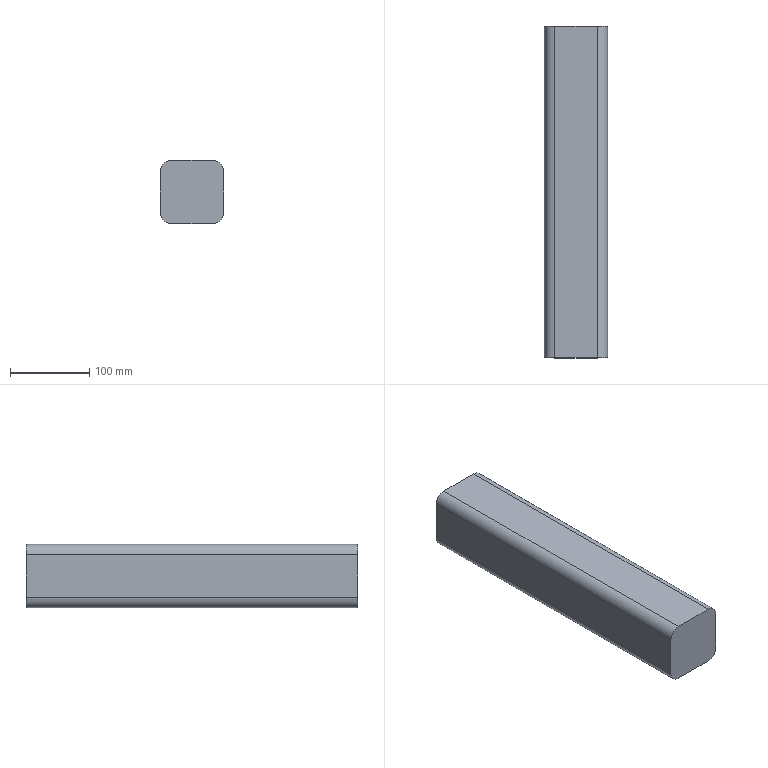Part | SolidWorks | features Extrusion 1 | 1 solid | 10 faces | box 80 x 420 x 80 mm | volume 2623906 mm3 | plane 6 | cylinder 4 | commonest cylinder face diameters 26.667 x4
STEP:
#1=CARTESIAN_POINT('',(26.667,0.,-40.));
#2=VERTEX_POINT('',#1);
#3=CARTESIAN_POINT('',(40.,0.,-26.667));
#4=VERTEX_POINT('',#3);
#5=CARTESIAN_POINT('',(26.667,0.,-26.667));
#6=DIRECTION('',(0.,-1.,0.));
#7=DIRECTION('',(0.,0.,-1.));
#8=AXIS2_PLACEMENT_3D('',#5,#6,#7);
#9=CIRCLE('',#8,13.333);
#10=EDGE_CURVE('',#2,#4,#9,.T.);
#11=ORIENTED_EDGE('',*,*,#10,.F.);
#12=CARTESIAN_POINT('',(26.667,420.,-40.));
#13=VERTEX_POINT('',#12);
#14=CARTESIAN_POINT('',(26.667,420.,-40.));
#15=DIRECTION('',(0.,-1.,0.));
#16=VECTOR('',#15,1000.);
#17=LINE('',#14,#16);
#18=EDGE_CURVE('',#13,#2,#17,.T.);
#19=ORIENTED_EDGE('',*,*,#18,.F.);
#20=CARTESIAN_POINT('',(40.,420.,-26.667));
#21=VERTEX_POINT('',#20);
#22=CARTESIAN_POINT('',(26.667,420.,-26.667));
#23=DIRECTION('',(0.,-1.,0.));
#24=DIRECTION('',(0.,0.,-1.));
#25=AXIS2_PLACEMENT_3D('',#22,#23,#24);
#26=CIRCLE('',#25,13.333);
#27=EDGE_CURVE('',#13,#21,#26,.T.);
#28=ORIENTED_EDGE('',*,*,#27,.T.);
#29=CARTESIAN_POINT('',(40.,420.,-26.667));
#30=DIRECTION('',(0.,-1.,0.));
#31=VECTOR('',#30,1000.);
#32=LINE('',#29,#31);
#33=EDGE_CURVE('',#21,#4,#32,.T.);
#34=ORIENTED_EDGE('',*,*,#33,.T.);
#35=EDGE_LOOP('',(#11,#19,#28,#34));
#36=FACE_OUTER_BOUND('',#35,.T.);
#37=CARTESIAN_POINT('',(26.667,420.,-26.667));
#38=DIRECTION('',(0.,-1.,0.));
#39=DIRECTION('',(0.,0.,-1.));
#40=AXIS2_PLACEMENT_3D('',#37,#38,#39);
#41=CYLINDRICAL_SURFACE('',#40,13.333);
#42=ADVANCED_FACE('',(#36),#41,.T.);
#43=CARTESIAN_POINT('',(-26.667,0.,-40.));
#44=VERTEX_POINT('',#43);
#45=CARTESIAN_POINT('',(-26.667,0.,-40.));
#46=DIRECTION('',(1.,0.,0.));
#47=VECTOR('',#46,1000.);
#48=LINE('',#45,#47);
#49=EDGE_CURVE('',#44,#2,#48,.T.);
#50=ORIENTED_EDGE('',*,*,#49,.F.);
#51=CARTESIAN_POINT('',(-26.667,420.,-40.));
#52=VERTEX_POINT('',#51);
#53=CARTESIAN_POINT('',(-26.667,420.,-40.));
#54=DIRECTION('',(0.,-1.,0.));
#55=VECTOR('',#54,1000.);
#56=LINE('',#53,#55);
#57=EDGE_CURVE('',#52,#44,#56,.T.);
#58=ORIENTED_EDGE('',*,*,#57,.F.);
#59=CARTESIAN_POINT('',(-26.667,420.,-40.));
#60=DIRECTION('',(1.,0.,0.));
#61=VECTOR('',#60,1000.);
#62=LINE('',#59,#61);
#63=EDGE_CURVE('',#52,#13,#62,.T.);
#64=ORIENTED_EDGE('',*,*,#63,.T.);
#65=ORIENTED_EDGE('',*,*,#18,.T.);
#66=EDGE_LOOP('',(#50,#58,#64,#65));
#67=FACE_OUTER_BOUND('',#66,.T.);
#68=CARTESIAN_POINT('',(-26.667,420.,-40.));
#69=DIRECTION('',(0.,0.,-1.));
#70=DIRECTION('',(0.,1.,0.));
#71=AXIS2_PLACEMENT_3D('',#68,#69,#70);
#72=PLANE('',#71);
#73=ADVANCED_FACE('',(#67),#72,.T.);
#74=CARTESIAN_POINT('',(-40.,0.,-26.667));
#75=VERTEX_POINT('',#74);
#76=CARTESIAN_POINT('',(-26.667,0.,-26.667));
#77=DIRECTION('',(0.,-1.,0.));
#78=DIRECTION('',(0.,0.,-1.));
#79=AXIS2_PLACEMENT_3D('',#76,#77,#78);
#80=CIRCLE('',#79,13.333);
#81=EDGE_CURVE('',#75,#44,#80,.T.);
#82=ORIENTED_EDGE('',*,*,#81,.F.);
#83=CARTESIAN_POINT('',(-40.,420.,-26.667));
#84=VERTEX_POINT('',#83);
#85=CARTESIAN_POINT('',(-40.,420.,-26.667));
#86=DIRECTION('',(0.,-1.,0.));
#87=VECTOR('',#86,1000.);
#88=LINE('',#85,#87);
#89=EDGE_CURVE('',#84,#75,#88,.T.);
#90=ORIENTED_EDGE('',*,*,#89,.F.);
#91=CARTESIAN_POINT('',(-26.667,420.,-26.667));
#92=DIRECTION('',(0.,-1.,0.));
#93=DIRECTION('',(0.,0.,-1.));
#94=AXIS2_PLACEMENT_3D('',#91,#92,#93);
#95=CIRCLE('',#94,13.333);
#96=EDGE_CURVE('',#84,#52,#95,.T.);
#97=ORIENTED_EDGE('',*,*,#96,.T.);
#98=ORIENTED_EDGE('',*,*,#57,.T.);
#99=EDGE_LOOP('',(#82,#90,#97,#98));
#100=FACE_OUTER_BOUND('',#99,.T.);
#101=CARTESIAN_POINT('',(-26.667,420.,-26.667));
#102=DIRECTION('',(0.,-1.,0.));
#103=DIRECTION('',(0.,0.,-1.));
#104=AXIS2_PLACEMENT_3D('',#101,#102,#103);
#105=CYLINDRICAL_SURFACE('',#104,13.333);
#106=ADVANCED_FACE('',(#100),#105,.T.);
#107=CARTESIAN_POINT('',(-40.,0.,26.667));
#108=VERTEX_POINT('',#107);
#109=CARTESIAN_POINT('',(-40.,0.,26.667));
#110=DIRECTION('',(0.,0.,-1.));
#111=VECTOR('',#110,1000.);
#112=LINE('',#109,#111);
#113=EDGE_CURVE('',#108,#75,#112,.T.);
#114=ORIENTED_EDGE('',*,*,#113,.F.);
#115=CARTESIAN_POINT('',(-40.,420.,26.667));
#116=VERTEX_POINT('',#115);
#117=CARTESIAN_POINT('',(-40.,420.,26.667));
#118=DIRECTION('',(0.,-1.,0.));
#119=VECTOR('',#118,1000.);
#120=LINE('',#117,#119);
#121=EDGE_CURVE('',#116,#108,#120,.T.);
#122=ORIENTED_EDGE('',*,*,#121,.F.);
#123=CARTESIAN_POINT('',(-40.,420.,26.667));
#124=DIRECTION('',(0.,0.,-1.));
#125=VECTOR('',#124,1000.);
#126=LINE('',#123,#125);
#127=EDGE_CURVE('',#116,#84,#126,.T.);
#128=ORIENTED_EDGE('',*,*,#127,.T.);
#129=ORIENTED_EDGE('',*,*,#89,.T.);
#130=EDGE_LOOP('',(#114,#122,#128,#129));
#131=FACE_OUTER_BOUND('',#130,.T.);
#132=CARTESIAN_POINT('',(-40.,420.,26.667));
#133=DIRECTION('',(-1.,0.,0.));
#134=DIRECTION('',(0.,0.,1.));
#135=AXIS2_PLACEMENT_3D('',#132,#133,#134);
#136=PLANE('',#135);
#137=ADVANCED_FACE('',(#131),#136,.T.);
#138=CARTESIAN_POINT('',(-26.667,0.,40.));
#139=VERTEX_POINT('',#138);
#140=CARTESIAN_POINT('',(-26.667,0.,26.667));
#141=DIRECTION('',(0.,-1.,0.));
#142=DIRECTION('',(0.,0.,-1.));
#143=AXIS2_PLACEMENT_3D('',#140,#141,#142);
#144=CIRCLE('',#143,13.333);
#145=EDGE_CURVE('',#139,#108,#144,.T.);
#146=ORIENTED_EDGE('',*,*,#145,.F.);
#147=CARTESIAN_POINT('',(-26.667,420.,40.));
#148=VERTEX_POINT('',#147);
#149=CARTESIAN_POINT('',(-26.667,420.,40.));
#150=DIRECTION('',(0.,-1.,0.));
#151=VECTOR('',#150,1000.);
#152=LINE('',#149,#151);
#153=EDGE_CURVE('',#148,#139,#152,.T.);
#154=ORIENTED_EDGE('',*,*,#153,.F.);
#155=CARTESIAN_POINT('',(-26.667,420.,26.667));
#156=DIRECTION('',(0.,-1.,0.));
#157=DIRECTION('',(0.,0.,-1.));
#158=AXIS2_PLACEMENT_3D('',#155,#156,#157);
#159=CIRCLE('',#158,13.333);
#160=EDGE_CURVE('',#148,#116,#159,.T.);
#161=ORIENTED_EDGE('',*,*,#160,.T.);
#162=ORIENTED_EDGE('',*,*,#121,.T.);
#163=EDGE_LOOP('',(#146,#154,#161,#162));
#164=FACE_OUTER_BOUND('',#163,.T.);
#165=CARTESIAN_POINT('',(-26.667,420.,26.667));
#166=DIRECTION('',(0.,-1.,0.));
#167=DIRECTION('',(0.,0.,-1.));
#168=AXIS2_PLACEMENT_3D('',#165,#166,#167);
#169=CYLINDRICAL_SURFACE('',#168,13.333);
#170=ADVANCED_FACE('',(#164),#169,.T.);
#171=CARTESIAN_POINT('',(26.667,0.,40.));
#172=VERTEX_POINT('',#171);
#173=CARTESIAN_POINT('',(26.667,0.,40.));
#174=DIRECTION('',(-1.,0.,0.));
#175=VECTOR('',#174,1000.);
#176=LINE('',#173,#175);
#177=EDGE_CURVE('',#172,#139,#176,.T.);
#178=ORIENTED_EDGE('',*,*,#177,.F.);
#179=CARTESIAN_POINT('',(26.667,420.,40.));
#180=VERTEX_POINT('',#179);
#181=CARTESIAN_POINT('',(26.667,420.,40.));
#182=DIRECTION('',(0.,-1.,0.));
#183=VECTOR('',#182,1000.);
#184=LINE('',#181,#183);
#185=EDGE_CURVE('',#180,#172,#184,.T.);
#186=ORIENTED_EDGE('',*,*,#185,.F.);
#187=CARTESIAN_POINT('',(26.667,420.,40.));
#188=DIRECTION('',(-1.,0.,0.));
#189=VECTOR('',#188,1000.);
#190=LINE('',#187,#189);
#191=EDGE_CURVE('',#180,#148,#190,.T.);
#192=ORIENTED_EDGE('',*,*,#191,.T.);
#193=ORIENTED_EDGE('',*,*,#153,.T.);
#194=EDGE_LOOP('',(#178,#186,#192,#193));
#195=FACE_OUTER_BOUND('',#194,.T.);
#196=CARTESIAN_POINT('',(26.667,420.,40.));
#197=DIRECTION('',(0.,0.,1.));
#198=DIRECTION('',(0.,-1.,0.));
#199=AXIS2_PLACEMENT_3D('',#196,#197,#198);
#200=PLANE('',#199);
#201=ADVANCED_FACE('',(#195),#200,.T.);
#202=CARTESIAN_POINT('',(40.,0.,26.667));
#203=VERTEX_POINT('',#202);
#204=CARTESIAN_POINT('',(26.667,0.,26.667));
#205=DIRECTION('',(0.,-1.,0.));
#206=DIRECTION('',(0.,0.,-1.));
#207=AXIS2_PLACEMENT_3D('',#204,#205,#206);
#208=CIRCLE('',#207,13.333);
#209=EDGE_CURVE('',#203,#172,#208,.T.);
#210=ORIENTED_EDGE('',*,*,#209,.F.);
#211=CARTESIAN_POINT('',(40.,420.,26.667));
#212=VERTEX_POINT('',#211);
#213=CARTESIAN_POINT('',(40.,420.,26.667));
#214=DIRECTION('',(0.,-1.,0.));
#215=VECTOR('',#214,1000.);
#216=LINE('',#213,#215);
#217=EDGE_CURVE('',#212,#203,#216,.T.);
#218=ORIENTED_EDGE('',*,*,#217,.F.);
#219=CARTESIAN_POINT('',(26.667,420.,26.667));
#220=DIRECTION('',(0.,-1.,0.));
#221=DIRECTION('',(0.,0.,-1.));
#222=AXIS2_PLACEMENT_3D('',#219,#220,#221);
#223=CIRCLE('',#222,13.333);
#224=EDGE_CURVE('',#212,#180,#223,.T.);
#225=ORIENTED_EDGE('',*,*,#224,.T.);
#226=ORIENTED_EDGE('',*,*,#185,.T.);
#227=EDGE_LOOP('',(#210,#218,#225,#226));
#228=FACE_OUTER_BOUND('',#227,.T.);
#229=CARTESIAN_POINT('',(26.667,420.,26.667));
#230=DIRECTION('',(0.,-1.,0.));
#231=DIRECTION('',(0.,0.,-1.));
#232=AXIS2_PLACEMENT_3D('',#229,#230,#231);
#233=CYLINDRICAL_SURFACE('',#232,13.333);
#234=ADVANCED_FACE('',(#228),#233,.T.);
#235=CARTESIAN_POINT('',(40.,0.,-26.667));
#236=DIRECTION('',(0.,0.,1.));
#237=VECTOR('',#236,1000.);
#238=LINE('',#235,#237);
#239=EDGE_CURVE('',#4,#203,#238,.T.);
#240=ORIENTED_EDGE('',*,*,#239,.F.);
#241=ORIENTED_EDGE('',*,*,#33,.F.);
#242=CARTESIAN_POINT('',(40.,420.,-26.667));
#243=DIRECTION('',(0.,0.,1.));
#244=VECTOR('',#243,1000.);
#245=LINE('',#242,#244);
#246=EDGE_CURVE('',#21,#212,#245,.T.);
#247=ORIENTED_EDGE('',*,*,#246,.T.);
#248=ORIENTED_EDGE('',*,*,#217,.T.);
#249=EDGE_LOOP('',(#240,#241,#247,#248));
#250=FACE_OUTER_BOUND('',#249,.T.);
#251=CARTESIAN_POINT('',(40.,420.,-26.667));
#252=DIRECTION('',(1.,0.,0.));
#253=DIRECTION('',(0.,0.,-1.));
#254=AXIS2_PLACEMENT_3D('',#251,#252,#253);
#255=PLANE('',#254);
#256=ADVANCED_FACE('',(#250),#255,.T.);
#257=ORIENTED_EDGE('',*,*,#27,.F.);
#258=ORIENTED_EDGE('',*,*,#63,.F.);
#259=ORIENTED_EDGE('',*,*,#96,.F.);
#260=ORIENTED_EDGE('',*,*,#127,.F.);
#261=ORIENTED_EDGE('',*,*,#160,.F.);
#262=ORIENTED_EDGE('',*,*,#191,.F.);
#263=ORIENTED_EDGE('',*,*,#224,.F.);
#264=ORIENTED_EDGE('',*,*,#246,.F.);
#265=EDGE_LOOP('',(#257,#258,#259,#260,#261,#262,#263,#264));
#266=FACE_OUTER_BOUND('',#265,.T.);
#267=CARTESIAN_POINT('',(26.667,420.,-26.667));
#268=DIRECTION('',(0.,-1.,0.));
#269=DIRECTION('',(0.,0.,-1.));
#270=AXIS2_PLACEMENT_3D('',#267,#268,#269);
#271=PLANE('',#270);
#272=ADVANCED_FACE('',(#266),#271,.F.);
#273=ORIENTED_EDGE('',*,*,#10,.T.);
#274=ORIENTED_EDGE('',*,*,#239,.T.);
#275=ORIENTED_EDGE('',*,*,#209,.T.);
#276=ORIENTED_EDGE('',*,*,#177,.T.);
#277=ORIENTED_EDGE('',*,*,#145,.T.);
#278=ORIENTED_EDGE('',*,*,#113,.T.);
#279=ORIENTED_EDGE('',*,*,#81,.T.);
#280=ORIENTED_EDGE('',*,*,#49,.T.);
#281=EDGE_LOOP('',(#273,#274,#275,#276,#277,#278,#279,#280));
#282=FACE_OUTER_BOUND('',#281,.T.);
#283=CARTESIAN_POINT('',(26.667,0.,-26.667));
#284=DIRECTION('',(0.,-1.,0.));
#285=DIRECTION('',(0.,0.,-1.));
#286=AXIS2_PLACEMENT_3D('',#283,#284,#285);
#287=PLANE('',#286);
#288=ADVANCED_FACE('',(#282),#287,.T.);
#289=CLOSED_SHELL('',(#42,#73,#106,#137,#170,#201,#234,#256,#272,#288));
#290=MANIFOLD_SOLID_BREP('',#289);
#291=CARTESIAN_POINT('',(0.,0.,0.));
#292=DIRECTION('',(0.,0.,1.));
#293=DIRECTION('',(1.,0.,0.));
#294=AXIS2_PLACEMENT_3D('',#291,#292,#293);
#295=(LENGTH_UNIT()NAMED_UNIT(*)SI_UNIT(.MILLI.,.METRE.));
#296=UNCERTAINTY_MEASURE_WITH_UNIT(LENGTH_MEASURE(0.00001),#295,'','');
#297=(NAMED_UNIT(*)PLANE_ANGLE_UNIT()SI_UNIT($,.RADIAN.));
#298=(NAMED_UNIT(*)SI_UNIT($,.STERADIAN.)SOLID_ANGLE_UNIT());
#299=(GEOMETRIC_REPRESENTATION_CONTEXT(3)GLOBAL_UNCERTAINTY_ASSIGNED_CONTEXT((#296))GLOBAL_UNIT_ASSIGNED_CONTEXT((#295,#297,#298))REPRESENTATION_CONTEXT('',''));
#300=ADVANCED_BREP_SHAPE_REPRESENTATION('',(#290,#294),#299);